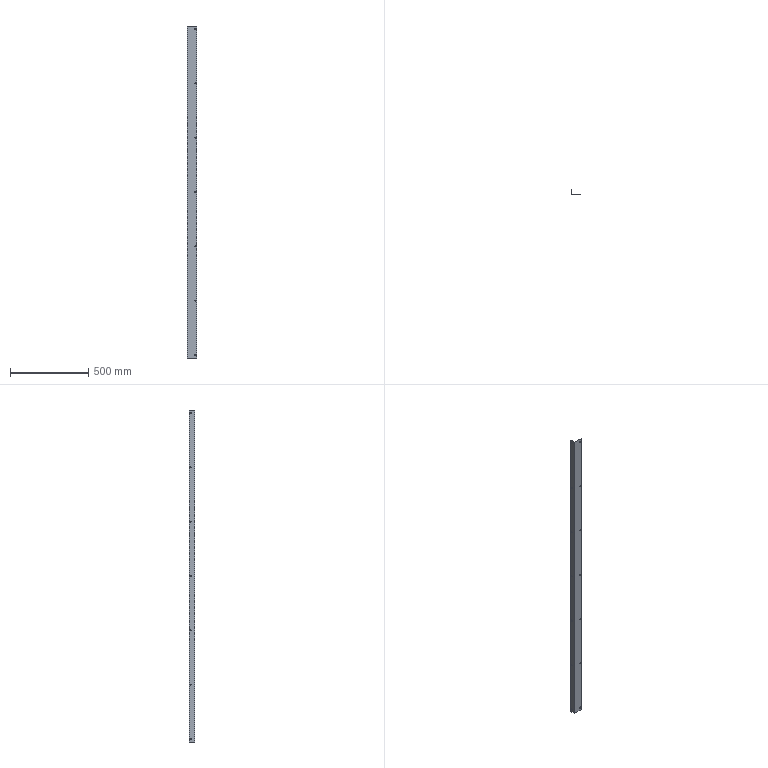Part | SolidWorks | features ICE 2, FlatPattern 1, SMBaseFlange 1, SheetMetal 1 | 1 solid | 70 faces | box 60 x 34 x 2116 mm | volume 195504 mm3 | plane 40 | cylinder 30 | commonest cylinder face diameters 6 x28 0.4 x1 2.4 x1